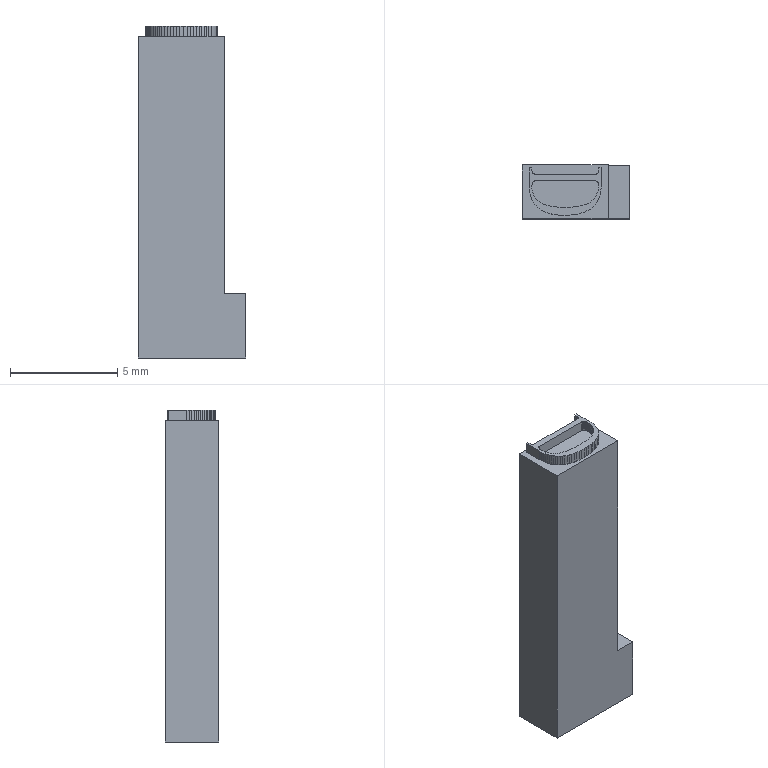Part | NX | features DIE-20 2 | 1 solid | 135 faces | box 5 x 2.5 x 15.5 mm | volume 158.702 mm3 | plane 135